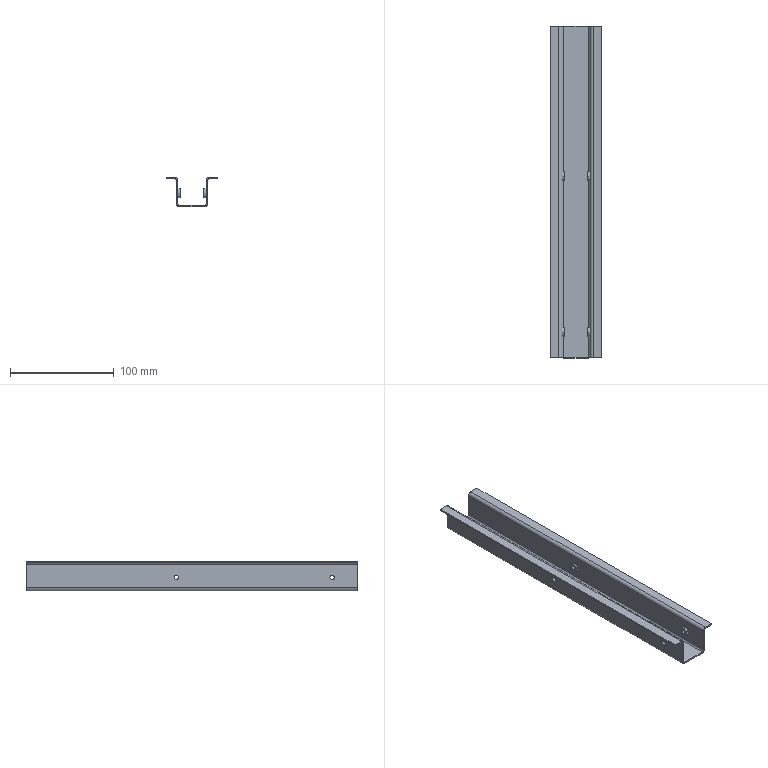Part | SolidWorks | features ICE 2, 3DProfileFeature 1, FlatPattern 1, HoleWzd 1, MirrorPattern 1, SMBaseFlange 1, SheetMetal 1 | 1 solid | 58 faces | box 50 x 320 x 28.5 mm | volume 48347 mm3 | plane 34 | cylinder 24 | commonest cylinder face diameters 4.2 x8 8.7 x8 3 x4 6 x4
STEP:
#1=CARTESIAN_POINT('',(-11.5,-225.,-11.9));
#2=VERTEX_POINT('',#1);
#3=CARTESIAN_POINT('',(-11.5,-225.,-16.1));
#4=VERTEX_POINT('',#3);
#5=CARTESIAN_POINT('',(-11.5,-225.,-14.));
#6=DIRECTION('',(1.,0.,0.));
#7=DIRECTION('',(0.,0.,-1.));
#8=AXIS2_PLACEMENT_3D('',#5,#6,#7);
#9=CIRCLE('',#8,2.1);
#10=EDGE_CURVE('',#2,#4,#9,.T.);
#11=ORIENTED_EDGE('',*,*,#10,.T.);
#12=CARTESIAN_POINT('',(-15.,-225.,-16.1));
#13=VERTEX_POINT('',#12);
#14=CARTESIAN_POINT('',(-15.,-225.,-16.1));
#15=DIRECTION('',(-1.,0.,0.));
#16=VECTOR('',#15,1000.);
#17=LINE('',#14,#16);
#18=EDGE_CURVE('',#4,#13,#17,.T.);
#19=ORIENTED_EDGE('',*,*,#18,.T.);
#20=CARTESIAN_POINT('',(-15.,-225.,-11.9));
#21=VERTEX_POINT('',#20);
#22=CARTESIAN_POINT('',(-15.,-225.,-14.));
#23=DIRECTION('',(-1.,0.,0.));
#24=DIRECTION('',(0.,0.,1.));
#25=AXIS2_PLACEMENT_3D('',#22,#23,#24);
#26=CIRCLE('',#25,2.1);
#27=EDGE_CURVE('',#13,#21,#26,.T.);
#28=ORIENTED_EDGE('',*,*,#27,.T.);
#29=CARTESIAN_POINT('',(-15.,-225.,-11.9));
#30=DIRECTION('',(-1.,0.,0.));
#31=VECTOR('',#30,1000.);
#32=LINE('',#29,#31);
#33=EDGE_CURVE('',#2,#21,#32,.T.);
#34=ORIENTED_EDGE('',*,*,#33,.F.);
#35=EDGE_LOOP('',(#11,#19,#28,#34));
#36=FACE_OUTER_BOUND('',#35,.T.);
#37=CARTESIAN_POINT('',(-15.,-225.,-14.));
#38=DIRECTION('',(-1.,0.,0.));
#39=DIRECTION('',(0.,0.,1.));
#40=AXIS2_PLACEMENT_3D('',#37,#38,#39);
#41=CYLINDRICAL_SURFACE('',#40,2.1);
#42=ADVANCED_FACE('',(#36),#41,.F.);
#43=CARTESIAN_POINT('',(15.,-225.,-11.9));
#44=VERTEX_POINT('',#43);
#45=CARTESIAN_POINT('',(15.,-225.,-16.1));
#46=VERTEX_POINT('',#45);
#47=CARTESIAN_POINT('',(15.,-225.,-14.));
#48=DIRECTION('',(1.,0.,0.));
#49=DIRECTION('',(0.,0.,-1.));
#50=AXIS2_PLACEMENT_3D('',#47,#48,#49);
#51=CIRCLE('',#50,2.1);
#52=EDGE_CURVE('',#44,#46,#51,.T.);
#53=ORIENTED_EDGE('',*,*,#52,.T.);
#54=CARTESIAN_POINT('',(11.5,-225.,-16.1));
#55=VERTEX_POINT('',#54);
#56=CARTESIAN_POINT('',(-15.,-225.,-16.1));
#57=DIRECTION('',(-1.,0.,0.));
#58=VECTOR('',#57,1000.);
#59=LINE('',#56,#58);
#60=EDGE_CURVE('',#46,#55,#59,.T.);
#61=ORIENTED_EDGE('',*,*,#60,.T.);
#62=CARTESIAN_POINT('',(11.5,-225.,-11.9));
#63=VERTEX_POINT('',#62);
#64=CARTESIAN_POINT('',(11.5,-225.,-14.));
#65=DIRECTION('',(-1.,0.,0.));
#66=DIRECTION('',(0.,0.,1.));
#67=AXIS2_PLACEMENT_3D('',#64,#65,#66);
#68=CIRCLE('',#67,2.1);
#69=EDGE_CURVE('',#55,#63,#68,.T.);
#70=ORIENTED_EDGE('',*,*,#69,.T.);
#71=CARTESIAN_POINT('',(-15.,-225.,-11.9));
#72=DIRECTION('',(-1.,0.,0.));
#73=VECTOR('',#72,1000.);
#74=LINE('',#71,#73);
#75=EDGE_CURVE('',#44,#63,#74,.T.);
#76=ORIENTED_EDGE('',*,*,#75,.F.);
#77=EDGE_LOOP('',(#53,#61,#70,#76));
#78=FACE_OUTER_BOUND('',#77,.T.);
#79=CARTESIAN_POINT('',(-15.,-225.,-14.));
#80=DIRECTION('',(-1.,0.,0.));
#81=DIRECTION('',(0.,0.,1.));
#82=AXIS2_PLACEMENT_3D('',#79,#80,#81);
#83=CYLINDRICAL_SURFACE('',#82,2.1);
#84=ADVANCED_FACE('',(#78),#83,.F.);
#85=CARTESIAN_POINT('',(15.,-75.,-11.9));
#86=VERTEX_POINT('',#85);
#87=CARTESIAN_POINT('',(15.,-75.,-16.1));
#88=VERTEX_POINT('',#87);
#89=CARTESIAN_POINT('',(15.,-75.,-14.));
#90=DIRECTION('',(1.,0.,0.));
#91=DIRECTION('',(0.,0.,-1.));
#92=AXIS2_PLACEMENT_3D('',#89,#90,#91);
#93=CIRCLE('',#92,2.1);
#94=EDGE_CURVE('',#86,#88,#93,.T.);
#95=ORIENTED_EDGE('',*,*,#94,.T.);
#96=CARTESIAN_POINT('',(11.5,-75.,-16.1));
#97=VERTEX_POINT('',#96);
#98=CARTESIAN_POINT('',(-15.,-75.,-16.1));
#99=DIRECTION('',(-1.,0.,0.));
#100=VECTOR('',#99,1000.);
#101=LINE('',#98,#100);
#102=EDGE_CURVE('',#88,#97,#101,.T.);
#103=ORIENTED_EDGE('',*,*,#102,.T.);
#104=CARTESIAN_POINT('',(11.5,-75.,-11.9));
#105=VERTEX_POINT('',#104);
#106=CARTESIAN_POINT('',(11.5,-75.,-14.));
#107=DIRECTION('',(1.,0.,0.));
#108=DIRECTION('',(0.,0.,-1.));
#109=AXIS2_PLACEMENT_3D('',#106,#107,#108);
#110=CIRCLE('',#109,2.1);
#111=EDGE_CURVE('',#105,#97,#110,.T.);
#112=ORIENTED_EDGE('',*,*,#111,.F.);
#113=CARTESIAN_POINT('',(-15.,-75.,-11.9));
#114=DIRECTION('',(-1.,0.,0.));
#115=VECTOR('',#114,1000.);
#116=LINE('',#113,#115);
#117=EDGE_CURVE('',#86,#105,#116,.T.);
#118=ORIENTED_EDGE('',*,*,#117,.F.);
#119=EDGE_LOOP('',(#95,#103,#112,#118));
#120=FACE_OUTER_BOUND('',#119,.T.);
#121=CARTESIAN_POINT('',(-15.,-75.,-14.));
#122=DIRECTION('',(-1.,0.,0.));
#123=DIRECTION('',(0.,0.,1.));
#124=AXIS2_PLACEMENT_3D('',#121,#122,#123);
#125=CYLINDRICAL_SURFACE('',#124,2.1);
#126=ADVANCED_FACE('',(#120),#125,.F.);
#127=CARTESIAN_POINT('',(-11.5,-75.,-16.1));
#128=VERTEX_POINT('',#127);
#129=CARTESIAN_POINT('',(-11.5,-75.,-11.9));
#130=VERTEX_POINT('',#129);
#131=CARTESIAN_POINT('',(-11.5,-75.,-14.));
#132=DIRECTION('',(-1.,0.,0.));
#133=DIRECTION('',(0.,0.,1.));
#134=AXIS2_PLACEMENT_3D('',#131,#132,#133);
#135=CIRCLE('',#134,2.1);
#136=EDGE_CURVE('',#128,#130,#135,.T.);
#137=ORIENTED_EDGE('',*,*,#136,.F.);
#138=CARTESIAN_POINT('',(-15.,-75.,-16.1));
#139=VERTEX_POINT('',#138);
#140=CARTESIAN_POINT('',(-15.,-75.,-16.1));
#141=DIRECTION('',(-1.,0.,0.));
#142=VECTOR('',#141,1000.);
#143=LINE('',#140,#142);
#144=EDGE_CURVE('',#128,#139,#143,.T.);
#145=ORIENTED_EDGE('',*,*,#144,.T.);
#146=CARTESIAN_POINT('',(-15.,-75.,-11.9));
#147=VERTEX_POINT('',#146);
#148=CARTESIAN_POINT('',(-15.,-75.,-14.));
#149=DIRECTION('',(-1.,0.,0.));
#150=DIRECTION('',(0.,0.,1.));
#151=AXIS2_PLACEMENT_3D('',#148,#149,#150);
#152=CIRCLE('',#151,2.1);
#153=EDGE_CURVE('',#139,#147,#152,.T.);
#154=ORIENTED_EDGE('',*,*,#153,.T.);
#155=CARTESIAN_POINT('',(-15.,-75.,-11.9));
#156=DIRECTION('',(-1.,0.,0.));
#157=VECTOR('',#156,1000.);
#158=LINE('',#155,#157);
#159=EDGE_CURVE('',#130,#147,#158,.T.);
#160=ORIENTED_EDGE('',*,*,#159,.F.);
#161=EDGE_LOOP('',(#137,#145,#154,#160));
#162=FACE_OUTER_BOUND('',#161,.T.);
#163=CARTESIAN_POINT('',(-15.,-75.,-14.));
#164=DIRECTION('',(-1.,0.,0.));
#165=DIRECTION('',(0.,0.,1.));
#166=AXIS2_PLACEMENT_3D('',#163,#164,#165);
#167=CYLINDRICAL_SURFACE('',#166,2.1);
#168=ADVANCED_FACE('',(#162),#167,.F.);
#169=CARTESIAN_POINT('',(11.5,-75.,-9.65));
#170=VERTEX_POINT('',#169);
#171=CARTESIAN_POINT('',(11.5,-75.,-18.35));
#172=VERTEX_POINT('',#171);
#173=CARTESIAN_POINT('',(11.5,-75.,-14.));
#174=DIRECTION('',(-1.,0.,0.));
#175=DIRECTION('',(0.,0.,1.));
#176=AXIS2_PLACEMENT_3D('',#173,#174,#175);
#177=CIRCLE('',#176,4.35);
#178=EDGE_CURVE('',#170,#172,#177,.T.);
#179=ORIENTED_EDGE('',*,*,#178,.F.);
#180=CARTESIAN_POINT('',(13.5,-75.,-9.65));
#181=VERTEX_POINT('',#180);
#182=CARTESIAN_POINT('',(11.5,-75.,-9.65));
#183=DIRECTION('',(1.,0.,0.));
#184=VECTOR('',#183,1000.);
#185=LINE('',#182,#184);
#186=EDGE_CURVE('',#170,#181,#185,.T.);
#187=ORIENTED_EDGE('',*,*,#186,.T.);
#188=CARTESIAN_POINT('',(13.5,-75.,-18.35));
#189=VERTEX_POINT('',#188);
#190=CARTESIAN_POINT('',(13.5,-75.,-14.));
#191=DIRECTION('',(-1.,0.,0.));
#192=DIRECTION('',(0.,0.,-1.));
#193=AXIS2_PLACEMENT_3D('',#190,#191,#192);
#194=CIRCLE('',#193,4.35);
#195=EDGE_CURVE('',#181,#189,#194,.T.);
#196=ORIENTED_EDGE('',*,*,#195,.T.);
#197=CARTESIAN_POINT('',(11.5,-75.,-18.35));
#198=DIRECTION('',(1.,0.,0.));
#199=VECTOR('',#198,1000.);
#200=LINE('',#197,#199);
#201=EDGE_CURVE('',#172,#189,#200,.T.);
#202=ORIENTED_EDGE('',*,*,#201,.F.);
#203=EDGE_LOOP('',(#179,#187,#196,#202));
#204=FACE_OUTER_BOUND('',#203,.T.);
#205=CARTESIAN_POINT('',(11.5,-75.,-14.));
#206=DIRECTION('',(1.,0.,0.));
#207=DIRECTION('',(0.,0.,-1.));
#208=AXIS2_PLACEMENT_3D('',#205,#206,#207);
#209=CYLINDRICAL_SURFACE('',#208,4.35);
#210=ADVANCED_FACE('',(#204),#209,.T.);
#211=CARTESIAN_POINT('',(11.5,-225.,-9.65));
#212=VERTEX_POINT('',#211);
#213=CARTESIAN_POINT('',(11.5,-225.,-18.35));
#214=VERTEX_POINT('',#213);
#215=CARTESIAN_POINT('',(11.5,-225.,-14.));
#216=DIRECTION('',(-1.,0.,0.));
#217=DIRECTION('',(0.,0.,-1.));
#218=AXIS2_PLACEMENT_3D('',#215,#216,#217);
#219=CIRCLE('',#218,4.35);
#220=EDGE_CURVE('',#212,#214,#219,.T.);
#221=ORIENTED_EDGE('',*,*,#220,.F.);
#222=CARTESIAN_POINT('',(13.5,-225.,-9.65));
#223=VERTEX_POINT('',#222);
#224=CARTESIAN_POINT('',(11.5,-225.,-9.65));
#225=DIRECTION('',(1.,0.,0.));
#226=VECTOR('',#225,1000.);
#227=LINE('',#224,#226);
#228=EDGE_CURVE('',#212,#223,#227,.T.);
#229=ORIENTED_EDGE('',*,*,#228,.T.);
#230=CARTESIAN_POINT('',(13.5,-225.,-18.35));
#231=VERTEX_POINT('',#230);
#232=CARTESIAN_POINT('',(13.5,-225.,-14.));
#233=DIRECTION('',(-1.,0.,0.));
#234=DIRECTION('',(0.,0.,-1.));
#235=AXIS2_PLACEMENT_3D('',#232,#233,#234);
#236=CIRCLE('',#235,4.35);
#237=EDGE_CURVE('',#223,#231,#236,.T.);
#238=ORIENTED_EDGE('',*,*,#237,.T.);
#239=CARTESIAN_POINT('',(11.5,-225.,-18.35));
#240=DIRECTION('',(1.,0.,0.));
#241=VECTOR('',#240,1000.);
#242=LINE('',#239,#241);
#243=EDGE_CURVE('',#214,#231,#242,.T.);
#244=ORIENTED_EDGE('',*,*,#243,.F.);
#245=EDGE_LOOP('',(#221,#229,#238,#244));
#246=FACE_OUTER_BOUND('',#245,.T.);
#247=CARTESIAN_POINT('',(11.5,-225.,-14.));
#248=DIRECTION('',(1.,0.,0.));
#249=DIRECTION('',(0.,0.,-1.));
#250=AXIS2_PLACEMENT_3D('',#247,#248,#249);
#251=CYLINDRICAL_SURFACE('',#250,4.35);
#252=ADVANCED_FACE('',(#246),#251,.T.);
#253=CARTESIAN_POINT('',(-11.5,-75.,-9.65));
#254=VERTEX_POINT('',#253);
#255=CARTESIAN_POINT('',(-11.5,-75.,-18.35));
#256=VERTEX_POINT('',#255);
#257=CARTESIAN_POINT('',(-11.5,-75.,-14.));
#258=DIRECTION('',(-1.,0.,0.));
#259=DIRECTION('',(0.,0.,1.));
#260=AXIS2_PLACEMENT_3D('',#257,#258,#259);
#261=CIRCLE('',#260,4.35);
#262=EDGE_CURVE('',#254,#256,#261,.T.);
#263=ORIENTED_EDGE('',*,*,#262,.T.);
#264=CARTESIAN_POINT('',(-13.5,-75.,-18.35));
#265=VERTEX_POINT('',#264);
#266=CARTESIAN_POINT('',(-11.5,-75.,-18.35));
#267=DIRECTION('',(-1.,0.,0.));
#268=VECTOR('',#267,1000.);
#269=LINE('',#266,#268);
#270=EDGE_CURVE('',#256,#265,#269,.T.);
#271=ORIENTED_EDGE('',*,*,#270,.T.);
#272=CARTESIAN_POINT('',(-13.5,-75.,-9.65));
#273=VERTEX_POINT('',#272);
#274=CARTESIAN_POINT('',(-13.5,-75.,-14.));
#275=DIRECTION('',(-1.,0.,0.));
#276=DIRECTION('',(0.,0.,1.));
#277=AXIS2_PLACEMENT_3D('',#274,#275,#276);
#278=CIRCLE('',#277,4.35);
#279=EDGE_CURVE('',#273,#265,#278,.T.);
#280=ORIENTED_EDGE('',*,*,#279,.F.);
#281=CARTESIAN_POINT('',(-11.5,-75.,-9.65));
#282=DIRECTION('',(-1.,0.,0.));
#283=VECTOR('',#282,1000.);
#284=LINE('',#281,#283);
#285=EDGE_CURVE('',#254,#273,#284,.T.);
#286=ORIENTED_EDGE('',*,*,#285,.F.);
#287=EDGE_LOOP('',(#263,#271,#280,#286));
#288=FACE_OUTER_BOUND('',#287,.T.);
#289=CARTESIAN_POINT('',(-11.5,-75.,-14.));
#290=DIRECTION('',(-1.,0.,0.));
#291=DIRECTION('',(0.,0.,1.));
#292=AXIS2_PLACEMENT_3D('',#289,#290,#291);
#293=CYLINDRICAL_SURFACE('',#292,4.35);
#294=ADVANCED_FACE('',(#288),#293,.T.);
#295=CARTESIAN_POINT('',(-11.5,-225.,-9.65));
#296=VERTEX_POINT('',#295);
#297=CARTESIAN_POINT('',(-11.5,-225.,-18.35));
#298=VERTEX_POINT('',#297);
#299=CARTESIAN_POINT('',(-11.5,-225.,-14.));
#300=DIRECTION('',(-1.,0.,0.));
#301=DIRECTION('',(0.,0.,-1.));
#302=AXIS2_PLACEMENT_3D('',#299,#300,#301);
#303=CIRCLE('',#302,4.35);
#304=EDGE_CURVE('',#296,#298,#303,.T.);
#305=ORIENTED_EDGE('',*,*,#304,.T.);
#306=CARTESIAN_POINT('',(-13.5,-225.,-18.35));
#307=VERTEX_POINT('',#306);
#308=CARTESIAN_POINT('',(-11.5,-225.,-18.35));
#309=DIRECTION('',(-1.,0.,0.));
#310=VECTOR('',#309,1000.);
#311=LINE('',#308,#310);
#312=EDGE_CURVE('',#298,#307,#311,.T.);
#313=ORIENTED_EDGE('',*,*,#312,.T.);
#314=CARTESIAN_POINT('',(-13.5,-225.,-9.65));
#315=VERTEX_POINT('',#314);
#316=CARTESIAN_POINT('',(-13.5,-225.,-14.));
#317=DIRECTION('',(-1.,0.,0.));
#318=DIRECTION('',(0.,0.,-1.));
#319=AXIS2_PLACEMENT_3D('',#316,#317,#318);
#320=CIRCLE('',#319,4.35);
#321=EDGE_CURVE('',#315,#307,#320,.T.);
#322=ORIENTED_EDGE('',*,*,#321,.F.);
#323=CARTESIAN_POINT('',(-11.5,-225.,-9.65));
#324=DIRECTION('',(-1.,0.,0.));
#325=VECTOR('',#324,1000.);
#326=LINE('',#323,#325);
#327=EDGE_CURVE('',#296,#315,#326,.T.);
#328=ORIENTED_EDGE('',*,*,#327,.F.);
#329=EDGE_LOOP('',(#305,#313,#322,#328));
#330=FACE_OUTER_BOUND('',#329,.T.);
#331=CARTESIAN_POINT('',(-11.5,-225.,-14.));
#332=DIRECTION('',(-1.,0.,0.));
#333=DIRECTION('',(0.,0.,1.));
#334=AXIS2_PLACEMENT_3D('',#331,#332,#333);
#335=CYLINDRICAL_SURFACE('',#334,4.35);
#336=ADVANCED_FACE('',(#330),#335,.T.);
#337=CARTESIAN_POINT('',(-16.5,70.,1.5));
#338=VERTEX_POINT('',#337);
#339=CARTESIAN_POINT('',(-25.,70.,1.5));
#340=VERTEX_POINT('',#339);
#341=CARTESIAN_POINT('',(-25.,70.,1.5));
#342=DIRECTION('',(-1.,0.,0.));
#343=VECTOR('',#342,1000.);
#344=LINE('',#341,#343);
#345=EDGE_CURVE('',#338,#340,#344,.T.);
#346=ORIENTED_EDGE('',*,*,#345,.F.);
#347=CARTESIAN_POINT('',(-16.5,70.,0.));
#348=VERTEX_POINT('',#347);
#349=CARTESIAN_POINT('',(-16.5,70.,1.5));
#350=DIRECTION('',(0.,0.,-1.));
#351=VECTOR('',#350,1000.);
#352=LINE('',#349,#351);
#353=EDGE_CURVE('',#338,#348,#352,.T.);
#354=ORIENTED_EDGE('',*,*,#353,.T.);
#355=CARTESIAN_POINT('',(-25.,70.,0.));
#356=VERTEX_POINT('',#355);
#357=CARTESIAN_POINT('',(-25.,70.,0.));
#358=DIRECTION('',(-1.,0.,0.));
#359=VECTOR('',#358,1000.);
#360=LINE('',#357,#359);
#361=EDGE_CURVE('',#348,#356,#360,.T.);
#362=ORIENTED_EDGE('',*,*,#361,.T.);
#363=CARTESIAN_POINT('',(-25.,70.,-43.176));
#364=DIRECTION('',(0.,0.,1.));
#365=VECTOR('',#364,1000.);
#366=LINE('',#363,#365);
#367=EDGE_CURVE('',#356,#340,#366,.T.);
#368=ORIENTED_EDGE('',*,*,#367,.T.);
#369=EDGE_LOOP('',(#346,#354,#362,#368));
#370=FACE_OUTER_BOUND('',#369,.T.);
#371=CARTESIAN_POINT('',(25.,70.,-43.176));
#372=DIRECTION('',(0.,-1.,0.));
#373=DIRECTION('',(0.,0.,-1.));
#374=AXIS2_PLACEMENT_3D('',#371,#372,#373);
#375=PLANE('',#374);
#376=ADVANCED_FACE('',(#370),#375,.F.);
#377=CARTESIAN_POINT('',(-15.,70.,-24.));
#378=VERTEX_POINT('',#377);
#379=CARTESIAN_POINT('',(-15.,70.,-1.5));
#380=VERTEX_POINT('',#379);
#381=CARTESIAN_POINT('',(-15.,70.,0.));
#382=DIRECTION('',(0.,0.,1.));
#383=VECTOR('',#382,1000.);
#384=LINE('',#381,#383);
#385=EDGE_CURVE('',#378,#380,#384,.T.);
#386=ORIENTED_EDGE('',*,*,#385,.T.);
#387=CARTESIAN_POINT('',(-13.5,70.,-1.5));
#388=VERTEX_POINT('',#387);
#389=CARTESIAN_POINT('',(-15.,70.,-1.5));
#390=DIRECTION('',(1.,0.,0.));
#391=VECTOR('',#390,1000.);
#392=LINE('',#389,#391);
#393=EDGE_CURVE('',#380,#388,#392,.T.);
#394=ORIENTED_EDGE('',*,*,#393,.T.);
#395=CARTESIAN_POINT('',(-13.5,70.,-24.));
#396=VERTEX_POINT('',#395);
#397=CARTESIAN_POINT('',(-13.5,70.,0.));
#398=DIRECTION('',(0.,0.,1.));
#399=VECTOR('',#398,1000.);
#400=LINE('',#397,#399);
#401=EDGE_CURVE('',#396,#388,#400,.T.);
#402=ORIENTED_EDGE('',*,*,#401,.F.);
#403=CARTESIAN_POINT('',(-13.5,70.,-24.));
#404=DIRECTION('',(-1.,0.,0.));
#405=VECTOR('',#404,1000.);
#406=LINE('',#403,#405);
#407=EDGE_CURVE('',#396,#378,#406,.T.);
#408=ORIENTED_EDGE('',*,*,#407,.T.);
#409=EDGE_LOOP('',(#386,#394,#402,#408));
#410=FACE_OUTER_BOUND('',#409,.T.);
#411=CARTESIAN_POINT('',(25.,70.,-43.176));
#412=DIRECTION('',(0.,-1.,0.));
#413=DIRECTION('',(0.,0.,-1.));
#414=AXIS2_PLACEMENT_3D('',#411,#412,#413);
#415=PLANE('',#414);
#416=ADVANCED_FACE('',(#410),#415,.F.);
#417=ORIENTED_EDGE('',*,*,#353,.F.);
#418=CARTESIAN_POINT('',(-16.5,70.,-1.5));
#419=DIRECTION('',(0.,-1.,0.));
#420=DIRECTION('',(0.,0.,-1.));
#421=AXIS2_PLACEMENT_3D('',#418,#419,#420);
#422=CIRCLE('',#421,3.);
#423=EDGE_CURVE('',#388,#338,#422,.T.);
#424=ORIENTED_EDGE('',*,*,#423,.F.);
#425=ORIENTED_EDGE('',*,*,#393,.F.);
#426=CARTESIAN_POINT('',(-16.5,70.,-1.5));
#427=DIRECTION('',(0.,-1.,0.));
#428=DIRECTION('',(0.,0.,-1.));
#429=AXIS2_PLACEMENT_3D('',#426,#427,#428);
#430=CIRCLE('',#429,1.5);
#431=EDGE_CURVE('',#380,#348,#430,.T.);
#432=ORIENTED_EDGE('',*,*,#431,.T.);
#433=EDGE_LOOP('',(#417,#424,#425,#432));
#434=FACE_OUTER_BOUND('',#433,.T.);
#435=CARTESIAN_POINT('',(25.,70.,-43.176));
#436=DIRECTION('',(0.,-1.,0.));
#437=DIRECTION('',(0.,0.,-1.));
#438=AXIS2_PLACEMENT_3D('',#435,#436,#437);
#439=PLANE('',#438);
#440=ADVANCED_FACE('',(#434),#439,.F.);
#441=CARTESIAN_POINT('',(12.,70.,-27.));
#442=VERTEX_POINT('',#441);
#443=CARTESIAN_POINT('',(-12.,70.,-27.));
#444=VERTEX_POINT('',#443);
#445=CARTESIAN_POINT('',(-15.,70.,-27.));
#446=DIRECTION('',(-1.,0.,0.));
#447=VECTOR('',#446,1000.);
#448=LINE('',#445,#447);
#449=EDGE_CURVE('',#442,#444,#448,.T.);
#450=ORIENTED_EDGE('',*,*,#449,.T.);
#451=CARTESIAN_POINT('',(-12.,70.,-25.5));
#452=VERTEX_POINT('',#451);
#453=CARTESIAN_POINT('',(-12.,70.,-27.));
#454=DIRECTION('',(0.,0.,1.));
#455=VECTOR('',#454,1000.);
#456=LINE('',#453,#455);
#457=EDGE_CURVE('',#444,#452,#456,.T.);
#458=ORIENTED_EDGE('',*,*,#457,.T.);
#459=CARTESIAN_POINT('',(12.,70.,-25.5));
#460=VERTEX_POINT('',#459);
#461=CARTESIAN_POINT('',(-15.,70.,-25.5));
#462=DIRECTION('',(-1.,0.,0.));
#463=VECTOR('',#462,1000.);
#464=LINE('',#461,#463);
#465=EDGE_CURVE('',#460,#452,#464,.T.);
#466=ORIENTED_EDGE('',*,*,#465,.F.);
#467=CARTESIAN_POINT('',(12.,70.,-25.5));
#468=DIRECTION('',(0.,0.,-1.));
#469=VECTOR('',#468,1000.);
#470=LINE('',#467,#469);
#471=EDGE_CURVE('',#460,#442,#470,.T.);
#472=ORIENTED_EDGE('',*,*,#471,.T.);
#473=EDGE_LOOP('',(#450,#458,#466,#472));
#474=FACE_OUTER_BOUND('',#473,.T.);
#475=CARTESIAN_POINT('',(25.,70.,-43.176));
#476=DIRECTION('',(0.,-1.,0.));
#477=DIRECTION('',(0.,0.,-1.));
#478=AXIS2_PLACEMENT_3D('',#475,#476,#477);
#479=PLANE('',#478);
#480=ADVANCED_FACE('',(#474),#479,.F.);
#481=ORIENTED_EDGE('',*,*,#407,.F.);
#482=CARTESIAN_POINT('',(-12.,70.,-24.));
#483=DIRECTION('',(0.,1.,0.));
#484=DIRECTION('',(0.,0.,-1.));
#485=AXIS2_PLACEMENT_3D('',#482,#483,#484);
#486=CIRCLE('',#485,1.5);
#487=EDGE_CURVE('',#452,#396,#486,.T.);
#488=ORIENTED_EDGE('',*,*,#487,.F.);
#489=ORIENTED_EDGE('',*,*,#457,.F.);
#490=CARTESIAN_POINT('',(-12.,70.,-24.));
#491=DIRECTION('',(0.,1.,0.));
#492=DIRECTION('',(0.,0.,-1.));
#493=AXIS2_PLACEMENT_3D('',#490,#491,#492);
#494=CIRCLE('',#493,3.);
#495=EDGE_CURVE('',#444,#378,#494,.T.);
#496=ORIENTED_EDGE('',*,*,#495,.T.);
#497=EDGE_LOOP('',(#481,#488,#489,#496));
#498=FACE_OUTER_BOUND('',#497,.T.);
#499=CARTESIAN_POINT('',(25.,70.,-43.176));
#500=DIRECTION('',(0.,-1.,0.));
#501=DIRECTION('',(0.,0.,-1.));
#502=AXIS2_PLACEMENT_3D('',#499,#500,#501);
#503=PLANE('',#502);
#504=ADVANCED_FACE('',(#498),#503,.F.);
#505=CARTESIAN_POINT('',(15.,70.,-1.5));
#506=VERTEX_POINT('',#505);
#507=CARTESIAN_POINT('',(15.,70.,-24.));
#508=VERTEX_POINT('',#507);
#509=CARTESIAN_POINT('',(15.,70.,-27.));
#510=DIRECTION('',(0.,0.,-1.));
#511=VECTOR('',#510,1000.);
#512=LINE('',#509,#511);
#513=EDGE_CURVE('',#506,#508,#512,.T.);
#514=ORIENTED_EDGE('',*,*,#513,.T.);
#515=CARTESIAN_POINT('',(13.5,70.,-24.));
#516=VERTEX_POINT('',#515);
#517=CARTESIAN_POINT('',(15.,70.,-24.));
#518=DIRECTION('',(-1.,0.,0.));
#519=VECTOR('',#518,1000.);
#520=LINE('',#517,#519);
#521=EDGE_CURVE('',#508,#516,#520,.T.);
#522=ORIENTED_EDGE('',*,*,#521,.T.);
#523=CARTESIAN_POINT('',(13.5,70.,-1.5));
#524=VERTEX_POINT('',#523);
#525=CARTESIAN_POINT('',(13.5,70.,-27.));
#526=DIRECTION('',(0.,0.,-1.));
#527=VECTOR('',#526,1000.);
#528=LINE('',#525,#527);
#529=EDGE_CURVE('',#524,#516,#528,.T.);
#530=ORIENTED_EDGE('',*,*,#529,.F.);
#531=CARTESIAN_POINT('',(13.5,70.,-1.5));
#532=DIRECTION('',(1.,0.,0.));
#533=VECTOR('',#532,1000.);
#534=LINE('',#531,#533);
#535=EDGE_CURVE('',#524,#506,#534,.T.);
#536=ORIENTED_EDGE('',*,*,#535,.T.);
#537=EDGE_LOOP('',(#514,#522,#530,#536));
#538=FACE_OUTER_BOUND('',#537,.T.);
#539=CARTESIAN_POINT('',(25.,70.,-43.176));
#540=DIRECTION('',(0.,-1.,0.));
#541=DIRECTION('',(0.,0.,-1.));
#542=AXIS2_PLACEMENT_3D('',#539,#540,#541);
#543=PLANE('',#542);
#544=ADVANCED_FACE('',(#538),#543,.F.);
#545=ORIENTED_EDGE('',*,*,#471,.F.);
#546=CARTESIAN_POINT('',(12.,70.,-24.));
#547=DIRECTION('',(0.,1.,0.));
#548=DIRECTION('',(0.,0.,-1.));
#549=AXIS2_PLACEMENT_3D('',#546,#547,#548);
#550=CIRCLE('',#549,1.5);
#551=EDGE_CURVE('',#516,#460,#550,.T.);
#552=ORIENTED_EDGE('',*,*,#551,.F.);
#553=ORIENTED_EDGE('',*,*,#521,.F.);
#554=CARTESIAN_POINT('',(12.,70.,-24.));
#555=DIRECTION('',(0.,1.,0.));
#556=DIRECTION('',(0.,0.,-1.));
#557=AXIS2_PLACEMENT_3D('',#554,#555,#556);
#558=CIRCLE('',#557,3.);
#559=EDGE_CURVE('',#508,#442,#558,.T.);
#560=ORIENTED_EDGE('',*,*,#559,.T.);
#561=EDGE_LOOP('',(#545,#552,#553,#560));
#562=FACE_OUTER_BOUND('',#561,.T.);
#563=CARTESIAN_POINT('',(25.,70.,-43.176));
#564=DIRECTION('',(0.,-1.,0.));
#565=DIRECTION('',(0.,0.,-1.));
#566=AXIS2_PLACEMENT_3D('',#563,#564,#565);
#567=PLANE('',#566);
#568=ADVANCED_FACE('',(#562),#567,.F.);
#569=CARTESIAN_POINT('',(25.,70.,0.));
#570=VERTEX_POINT('',#569);
#571=CARTESIAN_POINT('',(16.5,70.,0.));
#572=VERTEX_POINT('',#571);
#573=CARTESIAN_POINT('',(15.,70.,0.));
#574=DIRECTION('',(-1.,0.,0.));
#575=VECTOR('',#574,1000.);
#576=LINE('',#573,#575);
#577=EDGE_CURVE('',#570,#572,#576,.T.);
#578=ORIENTED_EDGE('',*,*,#577,.T.);
#579=CARTESIAN_POINT('',(16.5,70.,1.5));
#580=VERTEX_POINT('',#579);
#581=CARTESIAN_POINT('',(16.5,70.,0.));
#582=DIRECTION('',(0.,0.,1.));
#583=VECTOR('',#582,1000.);
#584=LINE('',#581,#583);
#585=EDGE_CURVE('',#572,#580,#584,.T.);
#586=ORIENTED_EDGE('',*,*,#585,.T.);
#587=CARTESIAN_POINT('',(25.,70.,1.5));
#588=VERTEX_POINT('',#587);
#589=CARTESIAN_POINT('',(15.,70.,1.5));
#590=DIRECTION('',(-1.,0.,0.));
#591=VECTOR('',#590,1000.);
#592=LINE('',#589,#591);
#593=EDGE_CURVE('',#588,#580,#592,.T.);
#594=ORIENTED_EDGE('',*,*,#593,.F.);
#595=CARTESIAN_POINT('',(25.,70.,-43.176));
#596=DIRECTION('',(0.,0.,1.));
#597=VECTOR('',#596,1000.);
#598=LINE('',#595,#597);
#599=EDGE_CURVE('',#570,#588,#598,.T.);
#600=ORIENTED_EDGE('',*,*,#599,.F.);
#601=EDGE_LOOP('',(#578,#586,#594,#600));
#602=FACE_OUTER_BOUND('',#601,.T.);
#603=CARTESIAN_POINT('',(25.,70.,-43.176));
#604=DIRECTION('',(0.,-1.,0.));
#605=DIRECTION('',(0.,0.,-1.));
#606=AXIS2_PLACEMENT_3D('',#603,#604,#605);
#607=PLANE('',#606);
#608=ADVANCED_FACE('',(#602),#607,.F.);
#609=CARTESIAN_POINT('',(-16.5,-250.,0.));
#610=VERTEX_POINT('',#609);
#611=CARTESIAN_POINT('',(-16.5,-250.,1.5));
#612=VERTEX_POINT('',#611);
#613=CARTESIAN_POINT('',(-16.5,-250.,0.));
#614=DIRECTION('',(0.,0.,1.));
#615=VECTOR('',#614,1000.);
#616=LINE('',#613,#615);
#617=EDGE_CURVE('',#610,#612,#616,.T.);
#618=ORIENTED_EDGE('',*,*,#617,.F.);
#619=CARTESIAN_POINT('',(-15.,-250.,-1.5));
#620=VERTEX_POINT('',#619);
#621=CARTESIAN_POINT('',(-16.5,-250.,-1.5));
#622=DIRECTION('',(0.,1.,0.));
#623=DIRECTION('',(0.,0.,-1.));
#624=AXIS2_PLACEMENT_3D('',#621,#622,#623);
#625=CIRCLE('',#624,1.5);
#626=EDGE_CURVE('',#610,#620,#625,.T.);
#627=ORIENTED_EDGE('',*,*,#626,.T.);
#628=CARTESIAN_POINT('',(-13.5,-250.,-1.5));
#629=VERTEX_POINT('',#628);
#630=CARTESIAN_POINT('',(-13.5,-250.,-1.5));
#631=DIRECTION('',(-1.,0.,0.));
#632=VECTOR('',#631,1000.);
#633=LINE('',#630,#632);
#634=EDGE_CURVE('',#629,#620,#633,.T.);
#635=ORIENTED_EDGE('',*,*,#634,.F.);
#636=CARTESIAN_POINT('',(-16.5,-250.,-1.5));
#637=DIRECTION('',(0.,1.,0.));
#638=DIRECTION('',(1.,0.,0.));
#639=AXIS2_PLACEMENT_3D('',#636,#637,#638);
#640=CIRCLE('',#639,3.);
#641=EDGE_CURVE('',#612,#629,#640,.T.);
#642=ORIENTED_EDGE('',*,*,#641,.F.);
#643=EDGE_LOOP('',(#618,#627,#635,#642));
#644=FACE_OUTER_BOUND('',#643,.T.);
#645=CARTESIAN_POINT('',(-16.5,-250.,0.));
#646=DIRECTION('',(0.,-1.,0.));
#647=DIRECTION('',(0.,0.,-1.));
#648=AXIS2_PLACEMENT_3D('',#645,#646,#647);
#649=PLANE('',#648);
#650=ADVANCED_FACE('',(#644),#649,.T.);
#651=CARTESIAN_POINT('',(-25.,-250.,0.));
#652=VERTEX_POINT('',#651);
#653=CARTESIAN_POINT('',(-25.,-250.,0.));
#654=DIRECTION('',(1.,0.,0.));
#655=VECTOR('',#654,1000.);
#656=LINE('',#653,#655);
#657=EDGE_CURVE('',#652,#610,#656,.T.);
#658=ORIENTED_EDGE('',*,*,#657,.T.);
#659=ORIENTED_EDGE('',*,*,#617,.T.);
#660=CARTESIAN_POINT('',(-25.,-250.,1.5));
#661=VERTEX_POINT('',#660);
#662=CARTESIAN_POINT('',(-25.,-250.,1.5));
#663=DIRECTION('',(1.,0.,0.));
#664=VECTOR('',#663,1000.);
#665=LINE('',#662,#664);
#666=EDGE_CURVE('',#661,#612,#665,.T.);
#667=ORIENTED_EDGE('',*,*,#666,.F.);
#668=CARTESIAN_POINT('',(-25.,-250.,1.5));
#669=DIRECTION('',(0.,0.,-1.));
#670=VECTOR('',#669,1000.);
#671=LINE('',#668,#670);
#672=EDGE_CURVE('',#661,#652,#671,.T.);
#673=ORIENTED_EDGE('',*,*,#672,.T.);
#674=EDGE_LOOP('',(#658,#659,#667,#673));
#675=FACE_OUTER_BOUND('',#674,.T.);
#676=CARTESIAN_POINT('',(-13.5,-250.,-1.5));
#677=DIRECTION('',(0.,-1.,0.));
#678=DIRECTION('',(0.,0.,-1.));
#679=AXIS2_PLACEMENT_3D('',#676,#677,#678);
#680=PLANE('',#679);
#681=ADVANCED_FACE('',(#675),#680,.T.);
#682=CARTESIAN_POINT('',(-15.,-250.,-24.));
#683=VERTEX_POINT('',#682);
#684=CARTESIAN_POINT('',(-13.5,-250.,-24.));
#685=VERTEX_POINT('',#684);
#686=CARTESIAN_POINT('',(-15.,-250.,-24.));
#687=DIRECTION('',(1.,0.,0.));
#688=VECTOR('',#687,1000.);
#689=LINE('',#686,#688);
#690=EDGE_CURVE('',#683,#685,#689,.T.);
#691=ORIENTED_EDGE('',*,*,#690,.F.);
#692=CARTESIAN_POINT('',(-12.,-250.,-27.));
#693=VERTEX_POINT('',#692);
#694=CARTESIAN_POINT('',(-12.,-250.,-24.));
#695=DIRECTION('',(0.,-1.,0.));
#696=DIRECTION('',(0.,0.,1.));
#697=AXIS2_PLACEMENT_3D('',#694,#695,#696);
#698=CIRCLE('',#697,3.);
#699=EDGE_CURVE('',#683,#693,#698,.T.);
#700=ORIENTED_EDGE('',*,*,#699,.T.);
#701=CARTESIAN_POINT('',(-12.,-250.,-25.5));
#702=VERTEX_POINT('',#701);
#703=CARTESIAN_POINT('',(-12.,-250.,-25.5));
#704=DIRECTION('',(0.,0.,-1.));
#705=VECTOR('',#704,1000.);
#706=LINE('',#703,#705);
#707=EDGE_CURVE('',#702,#693,#706,.T.);
#708=ORIENTED_EDGE('',*,*,#707,.F.);
#709=CARTESIAN_POINT('',(-12.,-250.,-24.));
#710=DIRECTION('',(0.,-1.,0.));
#711=DIRECTION('',(1.,0.,0.));
#712=AXIS2_PLACEMENT_3D('',#709,#710,#711);
#713=CIRCLE('',#712,1.5);
#714=EDGE_CURVE('',#685,#702,#713,.T.);
#715=ORIENTED_EDGE('',*,*,#714,.F.);
#716=EDGE_LOOP('',(#691,#700,#708,#715));
#717=FACE_OUTER_BOUND('',#716,.T.);
#718=CARTESIAN_POINT('',(-15.,-250.,-24.));
#719=DIRECTION('',(0.,-1.,0.));
#720=DIRECTION('',(0.,0.,-1.));
#721=AXIS2_PLACEMENT_3D('',#718,#719,#720);
#722=PLANE('',#721);
#723=ADVANCED_FACE('',(#717),#722,.T.);
#724=CARTESIAN_POINT('',(-15.,-250.,0.));
#725=DIRECTION('',(0.,0.,-1.));
#726=VECTOR('',#725,1000.);
#727=LINE('',#724,#726);
#728=EDGE_CURVE('',#620,#683,#727,.T.);
#729=ORIENTED_EDGE('',*,*,#728,.T.);
#730=ORIENTED_EDGE('',*,*,#690,.T.);
#731=CARTESIAN_POINT('',(-13.5,-250.,0.));
#732=DIRECTION('',(0.,0.,-1.));
#733=VECTOR('',#732,1000.);
#734=LINE('',#731,#733);
#735=EDGE_CURVE('',#629,#685,#734,.T.);
#736=ORIENTED_EDGE('',*,*,#735,.F.);
#737=ORIENTED_EDGE('',*,*,#634,.T.);
#738=EDGE_LOOP('',(#729,#730,#736,#737));
#739=FACE_OUTER_BOUND('',#738,.T.);
#740=CARTESIAN_POINT('',(-12.,-250.,-25.5));
#741=DIRECTION('',(0.,-1.,0.));
#742=DIRECTION('',(0.,0.,-1.));
#743=AXIS2_PLACEMENT_3D('',#740,#741,#742);
#744=PLANE('',#743);
#745=ADVANCED_FACE('',(#739),#744,.T.);
#746=CARTESIAN_POINT('',(12.,-250.,-27.));
#747=VERTEX_POINT('',#746);
#748=CARTESIAN_POINT('',(12.,-250.,-25.5));
#749=VERTEX_POINT('',#748);
#750=CARTESIAN_POINT('',(12.,-250.,-27.));
#751=DIRECTION('',(0.,0.,1.));
#752=VECTOR('',#751,1000.);
#753=LINE('',#750,#752);
#754=EDGE_CURVE('',#747,#749,#753,.T.);
#755=ORIENTED_EDGE('',*,*,#754,.F.);
#756=CARTESIAN_POINT('',(15.,-250.,-24.));
#757=VERTEX_POINT('',#756);
#758=CARTESIAN_POINT('',(12.,-250.,-24.));
#759=DIRECTION('',(0.,-1.,0.));
#760=DIRECTION('',(0.,0.,1.));
#761=AXIS2_PLACEMENT_3D('',#758,#759,#760);
#762=CIRCLE('',#761,3.);
#763=EDGE_CURVE('',#747,#757,#762,.T.);
#764=ORIENTED_EDGE('',*,*,#763,.T.);
#765=CARTESIAN_POINT('',(13.5,-250.,-24.));
#766=VERTEX_POINT('',#765);
#767=CARTESIAN_POINT('',(13.5,-250.,-24.));
#768=DIRECTION('',(1.,0.,0.));
#769=VECTOR('',#768,1000.);
#770=LINE('',#767,#769);
#771=EDGE_CURVE('',#766,#757,#770,.T.);
#772=ORIENTED_EDGE('',*,*,#771,.F.);
#773=CARTESIAN_POINT('',(12.,-250.,-24.));
#774=DIRECTION('',(0.,-1.,0.));
#775=DIRECTION('',(1.,0.,0.));
#776=AXIS2_PLACEMENT_3D('',#773,#774,#775);
#777=CIRCLE('',#776,1.5);
#778=EDGE_CURVE('',#749,#766,#777,.T.);
#779=ORIENTED_EDGE('',*,*,#778,.F.);
#780=EDGE_LOOP('',(#755,#764,#772,#779));
#781=FACE_OUTER_BOUND('',#780,.T.);
#782=CARTESIAN_POINT('',(12.,-250.,-27.));
#783=DIRECTION('',(0.,-1.,0.));
#784=DIRECTION('',(0.,0.,-1.));
#785=AXIS2_PLACEMENT_3D('',#782,#783,#784);
#786=PLANE('',#785);
#787=ADVANCED_FACE('',(#781),#786,.T.);
#788=CARTESIAN_POINT('',(-15.,-250.,-27.));
#789=DIRECTION('',(1.,0.,0.));
#790=VECTOR('',#789,1000.);
#791=LINE('',#788,#790);
#792=EDGE_CURVE('',#693,#747,#791,.T.);
#793=ORIENTED_EDGE('',*,*,#792,.T.);
#794=ORIENTED_EDGE('',*,*,#754,.T.);
#795=CARTESIAN_POINT('',(-15.,-250.,-25.5));
#796=DIRECTION('',(1.,0.,0.));
#797=VECTOR('',#796,1000.);
#798=LINE('',#795,#797);
#799=EDGE_CURVE('',#702,#749,#798,.T.);
#800=ORIENTED_EDGE('',*,*,#799,.F.);
#801=ORIENTED_EDGE('',*,*,#707,.T.);
#802=EDGE_LOOP('',(#793,#794,#800,#801));
#803=FACE_OUTER_BOUND('',#802,.T.);
#804=CARTESIAN_POINT('',(13.5,-250.,-24.));
#805=DIRECTION('',(0.,-1.,0.));
#806=DIRECTION('',(0.,0.,-1.));
#807=AXIS2_PLACEMENT_3D('',#804,#805,#806);
#808=PLANE('',#807);
#809=ADVANCED_FACE('',(#803),#808,.T.);
#810=CARTESIAN_POINT('',(15.,-250.,-1.5));
#811=VERTEX_POINT('',#810);
#812=CARTESIAN_POINT('',(13.5,-250.,-1.5));
#813=VERTEX_POINT('',#812);
#814=CARTESIAN_POINT('',(15.,-250.,-1.5));
#815=DIRECTION('',(-1.,0.,0.));
#816=VECTOR('',#815,1000.);
#817=LINE('',#814,#816);
#818=EDGE_CURVE('',#811,#813,#817,.T.);
#819=ORIENTED_EDGE('',*,*,#818,.F.);
#820=CARTESIAN_POINT('',(16.5,-250.,0.));
#821=VERTEX_POINT('',#820);
#822=CARTESIAN_POINT('',(16.5,-250.,-1.5));
#823=DIRECTION('',(0.,1.,0.));
#824=DIRECTION('',(0.,0.,-1.));
#825=AXIS2_PLACEMENT_3D('',#822,#823,#824);
#826=CIRCLE('',#825,1.5);
#827=EDGE_CURVE('',#811,#821,#826,.T.);
#828=ORIENTED_EDGE('',*,*,#827,.T.);
#829=CARTESIAN_POINT('',(16.5,-250.,1.5));
#830=VERTEX_POINT('',#829);
#831=CARTESIAN_POINT('',(16.5,-250.,1.5));
#832=DIRECTION('',(0.,0.,-1.));
#833=VECTOR('',#832,1000.);
#834=LINE('',#831,#833);
#835=EDGE_CURVE('',#830,#821,#834,.T.);
#836=ORIENTED_EDGE('',*,*,#835,.F.);
#837=CARTESIAN_POINT('',(16.5,-250.,-1.5));
#838=DIRECTION('',(0.,1.,0.));
#839=DIRECTION('',(1.,0.,0.));
#840=AXIS2_PLACEMENT_3D('',#837,#838,#839);
#841=CIRCLE('',#840,3.);
#842=EDGE_CURVE('',#813,#830,#841,.T.);
#843=ORIENTED_EDGE('',*,*,#842,.F.);
#844=EDGE_LOOP('',(#819,#828,#836,#843));
#845=FACE_OUTER_BOUND('',#844,.T.);
#846=CARTESIAN_POINT('',(15.,-250.,-1.5));
#847=DIRECTION('',(0.,-1.,0.));
#848=DIRECTION('',(0.,0.,-1.));
#849=AXIS2_PLACEMENT_3D('',#846,#847,#848);
#850=PLANE('',#849);
#851=ADVANCED_FACE('',(#845),#850,.T.);
#852=CARTESIAN_POINT('',(15.,-250.,-27.));
#853=DIRECTION('',(0.,0.,1.));
#854=VECTOR('',#853,1000.);
#855=LINE('',#852,#854);
#856=EDGE_CURVE('',#757,#811,#855,.T.);
#857=ORIENTED_EDGE('',*,*,#856,.T.);
#858=ORIENTED_EDGE('',*,*,#818,.T.);
#859=CARTESIAN_POINT('',(13.5,-250.,-27.));
#860=DIRECTION('',(0.,0.,1.));
#861=VECTOR('',#860,1000.);
#862=LINE('',#859,#861);
#863=EDGE_CURVE('',#766,#813,#862,.T.);
#864=ORIENTED_EDGE('',*,*,#863,.F.);
#865=ORIENTED_EDGE('',*,*,#771,.T.);
#866=EDGE_LOOP('',(#857,#858,#864,#865));
#867=FACE_OUTER_BOUND('',#866,.T.);
#868=CARTESIAN_POINT('',(16.5,-250.,1.5));
#869=DIRECTION('',(0.,-1.,0.));
#870=DIRECTION('',(0.,0.,-1.));
#871=AXIS2_PLACEMENT_3D('',#868,#869,#870);
#872=PLANE('',#871);
#873=ADVANCED_FACE('',(#867),#872,.T.);
#874=CARTESIAN_POINT('',(25.,-250.,1.5));
#875=VERTEX_POINT('',#874);
#876=CARTESIAN_POINT('',(25.,250.,1.5));
#877=DIRECTION('',(0.,-1.,0.));
#878=VECTOR('',#877,1000.);
#879=LINE('',#876,#878);
#880=EDGE_CURVE('',#588,#875,#879,.T.);
#881=ORIENTED_EDGE('',*,*,#880,.F.);
#882=ORIENTED_EDGE('',*,*,#593,.T.);
#883=CARTESIAN_POINT('',(16.5,250.,1.5));
#884=DIRECTION('',(0.,-1.,0.));
#885=VECTOR('',#884,1000.);
#886=LINE('',#883,#885);
#887=EDGE_CURVE('',#580,#830,#886,.T.);
#888=ORIENTED_EDGE('',*,*,#887,.T.);
#889=CARTESIAN_POINT('',(15.,-250.,1.5));
#890=DIRECTION('',(1.,0.,0.));
#891=VECTOR('',#890,1000.);
#892=LINE('',#889,#891);
#893=EDGE_CURVE('',#830,#875,#892,.T.);
#894=ORIENTED_EDGE('',*,*,#893,.T.);
#895=EDGE_LOOP('',(#881,#882,#888,#894));
#896=FACE_OUTER_BOUND('',#895,.T.);
#897=CARTESIAN_POINT('',(15.,250.,1.5));
#898=DIRECTION('',(0.,0.,-1.));
#899=DIRECTION('',(-1.,0.,0.));
#900=AXIS2_PLACEMENT_3D('',#897,#898,#899);
#901=PLANE('',#900);
#902=ADVANCED_FACE('',(#896),#901,.F.);
#903=ORIENTED_EDGE('',*,*,#599,.T.);
#904=ORIENTED_EDGE('',*,*,#880,.T.);
#905=CARTESIAN_POINT('',(25.,-250.,0.));
#906=VERTEX_POINT('',#905);
#907=CARTESIAN_POINT('',(25.,-250.,0.));
#908=DIRECTION('',(0.,0.,1.));
#909=VECTOR('',#908,1000.);
#910=LINE('',#907,#909);
#911=EDGE_CURVE('',#906,#875,#910,.T.);
#912=ORIENTED_EDGE('',*,*,#911,.F.);
#913=CARTESIAN_POINT('',(25.,250.,0.));
#914=DIRECTION('',(0.,-1.,0.));
#915=VECTOR('',#914,1000.);
#916=LINE('',#913,#915);
#917=EDGE_CURVE('',#570,#906,#916,.T.);
#918=ORIENTED_EDGE('',*,*,#917,.F.);
#919=EDGE_LOOP('',(#903,#904,#912,#918));
#920=FACE_OUTER_BOUND('',#919,.T.);
#921=CARTESIAN_POINT('',(25.,250.,0.));
#922=DIRECTION('',(1.,0.,0.));
#923=DIRECTION('',(0.,0.,-1.));
#924=AXIS2_PLACEMENT_3D('',#921,#922,#923);
#925=PLANE('',#924);
#926=ADVANCED_FACE('',(#920),#925,.T.);
#927=ORIENTED_EDGE('',*,*,#577,.F.);
#928=ORIENTED_EDGE('',*,*,#917,.T.);
#929=CARTESIAN_POINT('',(15.,-250.,0.));
#930=DIRECTION('',(1.,0.,0.));
#931=VECTOR('',#930,1000.);
#932=LINE('',#929,#931);
#933=EDGE_CURVE('',#821,#906,#932,.T.);
#934=ORIENTED_EDGE('',*,*,#933,.F.);
#935=CARTESIAN_POINT('',(16.5,250.,0.));
#936=DIRECTION('',(0.,-1.,0.));
#937=VECTOR('',#936,1000.);
#938=LINE('',#935,#937);
#939=EDGE_CURVE('',#572,#821,#938,.T.);
#940=ORIENTED_EDGE('',*,*,#939,.F.);
#941=EDGE_LOOP('',(#927,#928,#934,#940));
#942=FACE_OUTER_BOUND('',#941,.T.);
#943=CARTESIAN_POINT('',(15.,250.,0.));
#944=DIRECTION('',(0.,0.,-1.));
#945=DIRECTION('',(-1.,0.,0.));
#946=AXIS2_PLACEMENT_3D('',#943,#944,#945);
#947=PLANE('',#946);
#948=ADVANCED_FACE('',(#942),#947,.T.);
#949=CARTESIAN_POINT('',(16.5,70.,-1.5));
#950=DIRECTION('',(0.,-1.,0.));
#951=DIRECTION('',(0.,0.,-1.));
#952=AXIS2_PLACEMENT_3D('',#949,#950,#951);
#953=CIRCLE('',#952,1.5);
#954=EDGE_CURVE('',#572,#506,#953,.T.);
#955=ORIENTED_EDGE('',*,*,#954,.F.);
#956=ORIENTED_EDGE('',*,*,#939,.T.);
#957=ORIENTED_EDGE('',*,*,#827,.F.);
#958=CARTESIAN_POINT('',(15.,250.,-1.5));
#959=DIRECTION('',(0.,-1.,0.));
#960=VECTOR('',#959,1000.);
#961=LINE('',#958,#960);
#962=EDGE_CURVE('',#506,#811,#961,.T.);
#963=ORIENTED_EDGE('',*,*,#962,.F.);
#964=EDGE_LOOP('',(#955,#956,#957,#963));
#965=FACE_OUTER_BOUND('',#964,.T.);
#966=CARTESIAN_POINT('',(16.5,250.,-1.5));
#967=DIRECTION('',(0.,-1.,0.));
#968=DIRECTION('',(0.,0.,-1.));
#969=AXIS2_PLACEMENT_3D('',#966,#967,#968);
#970=CYLINDRICAL_SURFACE('',#969,1.5);
#971=ADVANCED_FACE('',(#965),#970,.F.);
#972=ORIENTED_EDGE('',*,*,#513,.F.);
#973=ORIENTED_EDGE('',*,*,#962,.T.);
#974=ORIENTED_EDGE('',*,*,#856,.F.);
#975=CARTESIAN_POINT('',(15.,250.,-24.));
#976=DIRECTION('',(0.,-1.,0.));
#977=VECTOR('',#976,1000.);
#978=LINE('',#975,#977);
#979=EDGE_CURVE('',#508,#757,#978,.T.);
#980=ORIENTED_EDGE('',*,*,#979,.F.);
#981=EDGE_LOOP('',(#972,#973,#974,#980));
#982=FACE_OUTER_BOUND('',#981,.T.);
#983=ORIENTED_EDGE('',*,*,#52,.F.);
#984=CARTESIAN_POINT('',(15.,-225.,-14.));
#985=DIRECTION('',(1.,0.,0.));
#986=DIRECTION('',(0.,0.,-1.));
#987=AXIS2_PLACEMENT_3D('',#984,#985,#986);
#988=CIRCLE('',#987,2.1);
#989=EDGE_CURVE('',#46,#44,#988,.T.);
#990=ORIENTED_EDGE('',*,*,#989,.F.);
#991=EDGE_LOOP('',(#983,#990));
#992=FACE_BOUND('',#991,.T.);
#993=ORIENTED_EDGE('',*,*,#94,.F.);
#994=CARTESIAN_POINT('',(15.,-75.,-14.));
#995=DIRECTION('',(1.,0.,0.));
#996=DIRECTION('',(0.,0.,-1.));
#997=AXIS2_PLACEMENT_3D('',#994,#995,#996);
#998=CIRCLE('',#997,2.1);
#999=EDGE_CURVE('',#88,#86,#998,.T.);
#1000=ORIENTED_EDGE('',*,*,#999,.F.);
#1001=EDGE_LOOP('',(#993,#1000));
#1002=FACE_BOUND('',#1001,.T.);
#1003=CARTESIAN_POINT('',(15.,250.,-27.));
#1004=DIRECTION('',(1.,0.,0.));
#1005=DIRECTION('',(0.,0.,-1.));
#1006=AXIS2_PLACEMENT_3D('',#1003,#1004,#1005);
#1007=PLANE('',#1006);
#1008=ADVANCED_FACE('',(#982,#992,#1002),#1007,.T.);
#1009=ORIENTED_EDGE('',*,*,#559,.F.);
#1010=ORIENTED_EDGE('',*,*,#979,.T.);
#1011=ORIENTED_EDGE('',*,*,#763,.F.);
#1012=CARTESIAN_POINT('',(12.,250.,-27.));
#1013=DIRECTION('',(0.,-1.,0.));
#1014=VECTOR('',#1013,1000.);
#1015=LINE('',#1012,#1014);
#1016=EDGE_CURVE('',#442,#747,#1015,.T.);
#1017=ORIENTED_EDGE('',*,*,#1016,.F.);
#1018=EDGE_LOOP('',(#1009,#1010,#1011,#1017));
#1019=FACE_OUTER_BOUND('',#1018,.T.);
#1020=CARTESIAN_POINT('',(12.,250.,-24.));
#1021=DIRECTION('',(0.,-1.,0.));
#1022=DIRECTION('',(0.,0.,-1.));
#1023=AXIS2_PLACEMENT_3D('',#1020,#1021,#1022);
#1024=CYLINDRICAL_SURFACE('',#1023,3.);
#1025=ADVANCED_FACE('',(#1019),#1024,.T.);
#1026=ORIENTED_EDGE('',*,*,#449,.F.);
#1027=ORIENTED_EDGE('',*,*,#1016,.T.);
#1028=ORIENTED_EDGE('',*,*,#792,.F.);
#1029=CARTESIAN_POINT('',(-12.,250.,-27.));
#1030=DIRECTION('',(0.,-1.,0.));
#1031=VECTOR('',#1030,1000.);
#1032=LINE('',#1029,#1031);
#1033=EDGE_CURVE('',#444,#693,#1032,.T.);
#1034=ORIENTED_EDGE('',*,*,#1033,.F.);
#1035=EDGE_LOOP('',(#1026,#1027,#1028,#1034));
#1036=FACE_OUTER_BOUND('',#1035,.T.);
#1037=CARTESIAN_POINT('',(-15.,250.,-27.));
#1038=DIRECTION('',(0.,0.,-1.));
#1039=DIRECTION('',(-1.,0.,0.));
#1040=AXIS2_PLACEMENT_3D('',#1037,#1038,#1039);
#1041=PLANE('',#1040);
#1042=ADVANCED_FACE('',(#1036),#1041,.T.);
#1043=ORIENTED_EDGE('',*,*,#495,.F.);
#1044=ORIENTED_EDGE('',*,*,#1033,.T.);
#1045=ORIENTED_EDGE('',*,*,#699,.F.);
#1046=CARTESIAN_POINT('',(-15.,250.,-24.));
#1047=DIRECTION('',(0.,-1.,0.));
#1048=VECTOR('',#1047,1000.);
#1049=LINE('',#1046,#1048);
#1050=EDGE_CURVE('',#378,#683,#1049,.T.);
#1051=ORIENTED_EDGE('',*,*,#1050,.F.);
#1052=EDGE_LOOP('',(#1043,#1044,#1045,#1051));
#1053=FACE_OUTER_BOUND('',#1052,.T.);
#1054=CARTESIAN_POINT('',(-12.,250.,-24.));
#1055=DIRECTION('',(0.,-1.,0.));
#1056=DIRECTION('',(0.,0.,-1.));
#1057=AXIS2_PLACEMENT_3D('',#1054,#1055,#1056);
#1058=CYLINDRICAL_SURFACE('',#1057,3.);
#1059=ADVANCED_FACE('',(#1053),#1058,.T.);
#1060=ORIENTED_EDGE('',*,*,#385,.F.);
#1061=ORIENTED_EDGE('',*,*,#1050,.T.);
#1062=ORIENTED_EDGE('',*,*,#728,.F.);
#1063=CARTESIAN_POINT('',(-15.,250.,-1.5));
#1064=DIRECTION('',(0.,-1.,0.));
#1065=VECTOR('',#1064,1000.);
#1066=LINE('',#1063,#1065);
#1067=EDGE_CURVE('',#380,#620,#1066,.T.);
#1068=ORIENTED_EDGE('',*,*,#1067,.F.);
#1069=EDGE_LOOP('',(#1060,#1061,#1062,#1068));
#1070=FACE_OUTER_BOUND('',#1069,.T.);
#1071=CARTESIAN_POINT('',(-15.,-225.,-14.));
#1072=DIRECTION('',(-1.,0.,0.));
#1073=DIRECTION('',(0.,0.,1.));
#1074=AXIS2_PLACEMENT_3D('',#1071,#1072,#1073);
#1075=CIRCLE('',#1074,2.1);
#1076=EDGE_CURVE('',#21,#13,#1075,.T.);
#1077=ORIENTED_EDGE('',*,*,#1076,.F.);
#1078=ORIENTED_EDGE('',*,*,#27,.F.);
#1079=EDGE_LOOP('',(#1077,#1078));
#1080=FACE_BOUND('',#1079,.T.);
#1081=CARTESIAN_POINT('',(-15.,-75.,-14.));
#1082=DIRECTION('',(-1.,0.,0.));
#1083=DIRECTION('',(0.,0.,1.));
#1084=AXIS2_PLACEMENT_3D('',#1081,#1082,#1083);
#1085=CIRCLE('',#1084,2.1);
#1086=EDGE_CURVE('',#147,#139,#1085,.T.);
#1087=ORIENTED_EDGE('',*,*,#1086,.F.);
#1088=ORIENTED_EDGE('',*,*,#153,.F.);
#1089=EDGE_LOOP('',(#1087,#1088));
#1090=FACE_BOUND('',#1089,.T.);
#1091=CARTESIAN_POINT('',(-15.,250.,0.));
#1092=DIRECTION('',(-1.,0.,0.));
#1093=DIRECTION('',(0.,0.,1.));
#1094=AXIS2_PLACEMENT_3D('',#1091,#1092,#1093);
#1095=PLANE('',#1094);
#1096=ADVANCED_FACE('',(#1070,#1080,#1090),#1095,.T.);
#1097=ORIENTED_EDGE('',*,*,#431,.F.);
#1098=ORIENTED_EDGE('',*,*,#1067,.T.);
#1099=ORIENTED_EDGE('',*,*,#626,.F.);
#1100=CARTESIAN_POINT('',(-16.5,250.,0.));
#1101=DIRECTION('',(0.,-1.,0.));
#1102=VECTOR('',#1101,1000.);
#1103=LINE('',#1100,#1102);
#1104=EDGE_CURVE('',#348,#610,#1103,.T.);
#1105=ORIENTED_EDGE('',*,*,#1104,.F.);
#1106=EDGE_LOOP('',(#1097,#1098,#1099,#1105));
#1107=FACE_OUTER_BOUND('',#1106,.T.);
#1108=CARTESIAN_POINT('',(-16.5,250.,-1.5));
#1109=DIRECTION('',(0.,-1.,0.));
#1110=DIRECTION('',(0.,0.,-1.));
#1111=AXIS2_PLACEMENT_3D('',#1108,#1109,#1110);
#1112=CYLINDRICAL_SURFACE('',#1111,1.5);
#1113=ADVANCED_FACE('',(#1107),#1112,.F.);
#1114=ORIENTED_EDGE('',*,*,#361,.F.);
#1115=ORIENTED_EDGE('',*,*,#1104,.T.);
#1116=ORIENTED_EDGE('',*,*,#657,.F.);
#1117=CARTESIAN_POINT('',(-25.,250.,0.));
#1118=DIRECTION('',(0.,-1.,0.));
#1119=VECTOR('',#1118,1000.);
#1120=LINE('',#1117,#1119);
#1121=EDGE_CURVE('',#356,#652,#1120,.T.);
#1122=ORIENTED_EDGE('',*,*,#1121,.F.);
#1123=EDGE_LOOP('',(#1114,#1115,#1116,#1122));
#1124=FACE_OUTER_BOUND('',#1123,.T.);
#1125=CARTESIAN_POINT('',(-25.,250.,0.));
#1126=DIRECTION('',(0.,0.,-1.));
#1127=DIRECTION('',(-1.,0.,0.));
#1128=AXIS2_PLACEMENT_3D('',#1125,#1126,#1127);
#1129=PLANE('',#1128);
#1130=ADVANCED_FACE('',(#1124),#1129,.T.);
#1131=ORIENTED_EDGE('',*,*,#367,.F.);
#1132=ORIENTED_EDGE('',*,*,#1121,.T.);
#1133=ORIENTED_EDGE('',*,*,#672,.F.);
#1134=CARTESIAN_POINT('',(-25.,250.,1.5));
#1135=DIRECTION('',(0.,-1.,0.));
#1136=VECTOR('',#1135,1000.);
#1137=LINE('',#1134,#1136);
#1138=EDGE_CURVE('',#340,#661,#1137,.T.);
#1139=ORIENTED_EDGE('',*,*,#1138,.F.);
#1140=EDGE_LOOP('',(#1131,#1132,#1133,#1139));
#1141=FACE_OUTER_BOUND('',#1140,.T.);
#1142=CARTESIAN_POINT('',(-25.,250.,1.5));
#1143=DIRECTION('',(-1.,0.,0.));
#1144=DIRECTION('',(0.,0.,1.));
#1145=AXIS2_PLACEMENT_3D('',#1142,#1143,#1144);
#1146=PLANE('',#1145);
#1147=ADVANCED_FACE('',(#1141),#1146,.T.);
#1148=CARTESIAN_POINT('',(-16.5,250.,1.5));
#1149=DIRECTION('',(0.,-1.,0.));
#1150=VECTOR('',#1149,1000.);
#1151=LINE('',#1148,#1150);
#1152=EDGE_CURVE('',#338,#612,#1151,.T.);
#1153=ORIENTED_EDGE('',*,*,#1152,.F.);
#1154=ORIENTED_EDGE('',*,*,#345,.T.);
#1155=ORIENTED_EDGE('',*,*,#1138,.T.);
#1156=ORIENTED_EDGE('',*,*,#666,.T.);
#1157=EDGE_LOOP('',(#1153,#1154,#1155,#1156));
#1158=FACE_OUTER_BOUND('',#1157,.T.);
#1159=CARTESIAN_POINT('',(-25.,250.,1.5));
#1160=DIRECTION('',(0.,0.,-1.));
#1161=DIRECTION('',(-1.,0.,0.));
#1162=AXIS2_PLACEMENT_3D('',#1159,#1160,#1161);
#1163=PLANE('',#1162);
#1164=ADVANCED_FACE('',(#1158),#1163,.F.);
#1165=CARTESIAN_POINT('',(-13.5,250.,-1.5));
#1166=DIRECTION('',(0.,-1.,0.));
#1167=VECTOR('',#1166,1000.);
#1168=LINE('',#1165,#1167);
#1169=EDGE_CURVE('',#388,#629,#1168,.T.);
#1170=ORIENTED_EDGE('',*,*,#1169,.F.);
#1171=ORIENTED_EDGE('',*,*,#423,.T.);
#1172=ORIENTED_EDGE('',*,*,#1152,.T.);
#1173=ORIENTED_EDGE('',*,*,#641,.T.);
#1174=EDGE_LOOP('',(#1170,#1171,#1172,#1173));
#1175=FACE_OUTER_BOUND('',#1174,.T.);
#1176=CARTESIAN_POINT('',(-16.5,250.,-1.5));
#1177=DIRECTION('',(0.,-1.,0.));
#1178=DIRECTION('',(0.,0.,-1.));
#1179=AXIS2_PLACEMENT_3D('',#1176,#1177,#1178);
#1180=CYLINDRICAL_SURFACE('',#1179,3.);
#1181=ADVANCED_FACE('',(#1175),#1180,.T.);
#1182=ORIENTED_EDGE('',*,*,#279,.T.);
#1183=CARTESIAN_POINT('',(-13.5,-75.,-14.));
#1184=DIRECTION('',(-1.,0.,0.));
#1185=DIRECTION('',(0.,0.,1.));
#1186=AXIS2_PLACEMENT_3D('',#1183,#1184,#1185);
#1187=CIRCLE('',#1186,4.35);
#1188=EDGE_CURVE('',#265,#273,#1187,.T.);
#1189=ORIENTED_EDGE('',*,*,#1188,.T.);
#1190=EDGE_LOOP('',(#1182,#1189));
#1191=FACE_BOUND('',#1190,.T.);
#1192=ORIENTED_EDGE('',*,*,#321,.T.);
#1193=CARTESIAN_POINT('',(-13.5,-225.,-14.));
#1194=DIRECTION('',(-1.,0.,0.));
#1195=DIRECTION('',(0.,0.,-1.));
#1196=AXIS2_PLACEMENT_3D('',#1193,#1194,#1195);
#1197=CIRCLE('',#1196,4.35);
#1198=EDGE_CURVE('',#307,#315,#1197,.T.);
#1199=ORIENTED_EDGE('',*,*,#1198,.T.);
#1200=EDGE_LOOP('',(#1192,#1199));
#1201=FACE_BOUND('',#1200,.T.);
#1202=CARTESIAN_POINT('',(-13.5,250.,-24.));
#1203=DIRECTION('',(0.,-1.,0.));
#1204=VECTOR('',#1203,1000.);
#1205=LINE('',#1202,#1204);
#1206=EDGE_CURVE('',#396,#685,#1205,.T.);
#1207=ORIENTED_EDGE('',*,*,#1206,.F.);
#1208=ORIENTED_EDGE('',*,*,#401,.T.);
#1209=ORIENTED_EDGE('',*,*,#1169,.T.);
#1210=ORIENTED_EDGE('',*,*,#735,.T.);
#1211=EDGE_LOOP('',(#1207,#1208,#1209,#1210));
#1212=FACE_OUTER_BOUND('',#1211,.T.);
#1213=CARTESIAN_POINT('',(-13.5,250.,0.));
#1214=DIRECTION('',(-1.,0.,0.));
#1215=DIRECTION('',(0.,0.,1.));
#1216=AXIS2_PLACEMENT_3D('',#1213,#1214,#1215);
#1217=PLANE('',#1216);
#1218=ADVANCED_FACE('',(#1191,#1201,#1212),#1217,.F.);
#1219=CARTESIAN_POINT('',(-12.,250.,-25.5));
#1220=DIRECTION('',(0.,-1.,0.));
#1221=VECTOR('',#1220,1000.);
#1222=LINE('',#1219,#1221);
#1223=EDGE_CURVE('',#452,#702,#1222,.T.);
#1224=ORIENTED_EDGE('',*,*,#1223,.F.);
#1225=ORIENTED_EDGE('',*,*,#487,.T.);
#1226=ORIENTED_EDGE('',*,*,#1206,.T.);
#1227=ORIENTED_EDGE('',*,*,#714,.T.);
#1228=EDGE_LOOP('',(#1224,#1225,#1226,#1227));
#1229=FACE_OUTER_BOUND('',#1228,.T.);
#1230=CARTESIAN_POINT('',(-12.,250.,-24.));
#1231=DIRECTION('',(0.,-1.,0.));
#1232=DIRECTION('',(0.,0.,-1.));
#1233=AXIS2_PLACEMENT_3D('',#1230,#1231,#1232);
#1234=CYLINDRICAL_SURFACE('',#1233,1.5);
#1235=ADVANCED_FACE('',(#1229),#1234,.F.);
#1236=CARTESIAN_POINT('',(12.,250.,-25.5));
#1237=DIRECTION('',(0.,-1.,0.));
#1238=VECTOR('',#1237,1000.);
#1239=LINE('',#1236,#1238);
#1240=EDGE_CURVE('',#460,#749,#1239,.T.);
#1241=ORIENTED_EDGE('',*,*,#1240,.F.);
#1242=ORIENTED_EDGE('',*,*,#465,.T.);
#1243=ORIENTED_EDGE('',*,*,#1223,.T.);
#1244=ORIENTED_EDGE('',*,*,#799,.T.);
#1245=EDGE_LOOP('',(#1241,#1242,#1243,#1244));
#1246=FACE_OUTER_BOUND('',#1245,.T.);
#1247=CARTESIAN_POINT('',(-15.,250.,-25.5));
#1248=DIRECTION('',(0.,0.,-1.));
#1249=DIRECTION('',(-1.,0.,0.));
#1250=AXIS2_PLACEMENT_3D('',#1247,#1248,#1249);
#1251=PLANE('',#1250);
#1252=ADVANCED_FACE('',(#1246),#1251,.F.);
#1253=CARTESIAN_POINT('',(13.5,250.,-24.));
#1254=DIRECTION('',(0.,-1.,0.));
#1255=VECTOR('',#1254,1000.);
#1256=LINE('',#1253,#1255);
#1257=EDGE_CURVE('',#516,#766,#1256,.T.);
#1258=ORIENTED_EDGE('',*,*,#1257,.F.);
#1259=ORIENTED_EDGE('',*,*,#551,.T.);
#1260=ORIENTED_EDGE('',*,*,#1240,.T.);
#1261=ORIENTED_EDGE('',*,*,#778,.T.);
#1262=EDGE_LOOP('',(#1258,#1259,#1260,#1261));
#1263=FACE_OUTER_BOUND('',#1262,.T.);
#1264=CARTESIAN_POINT('',(12.,250.,-24.));
#1265=DIRECTION('',(0.,-1.,0.));
#1266=DIRECTION('',(0.,0.,-1.));
#1267=AXIS2_PLACEMENT_3D('',#1264,#1265,#1266);
#1268=CYLINDRICAL_SURFACE('',#1267,1.5);
#1269=ADVANCED_FACE('',(#1263),#1268,.F.);
#1270=CARTESIAN_POINT('',(13.5,-75.,-14.));
#1271=DIRECTION('',(-1.,0.,0.));
#1272=DIRECTION('',(0.,0.,-1.));
#1273=AXIS2_PLACEMENT_3D('',#1270,#1271,#1272);
#1274=CIRCLE('',#1273,4.35);
#1275=EDGE_CURVE('',#189,#181,#1274,.T.);
#1276=ORIENTED_EDGE('',*,*,#1275,.F.);
#1277=ORIENTED_EDGE('',*,*,#195,.F.);
#1278=EDGE_LOOP('',(#1276,#1277));
#1279=FACE_BOUND('',#1278,.T.);
#1280=CARTESIAN_POINT('',(13.5,-225.,-14.));
#1281=DIRECTION('',(-1.,0.,0.));
#1282=DIRECTION('',(0.,0.,-1.));
#1283=AXIS2_PLACEMENT_3D('',#1280,#1281,#1282);
#1284=CIRCLE('',#1283,4.35);
#1285=EDGE_CURVE('',#231,#223,#1284,.T.);
#1286=ORIENTED_EDGE('',*,*,#1285,.F.);
#1287=ORIENTED_EDGE('',*,*,#237,.F.);
#1288=EDGE_LOOP('',(#1286,#1287));
#1289=FACE_BOUND('',#1288,.T.);
#1290=CARTESIAN_POINT('',(13.5,250.,-1.5));
#1291=DIRECTION('',(0.,-1.,0.));
#1292=VECTOR('',#1291,1000.);
#1293=LINE('',#1290,#1292);
#1294=EDGE_CURVE('',#524,#813,#1293,.T.);
#1295=ORIENTED_EDGE('',*,*,#1294,.F.);
#1296=ORIENTED_EDGE('',*,*,#529,.T.);
#1297=ORIENTED_EDGE('',*,*,#1257,.T.);
#1298=ORIENTED_EDGE('',*,*,#863,.T.);
#1299=EDGE_LOOP('',(#1295,#1296,#1297,#1298));
#1300=FACE_OUTER_BOUND('',#1299,.T.);
#1301=CARTESIAN_POINT('',(13.5,250.,-27.));
#1302=DIRECTION('',(1.,0.,0.));
#1303=DIRECTION('',(0.,0.,-1.));
#1304=AXIS2_PLACEMENT_3D('',#1301,#1302,#1303);
#1305=PLANE('',#1304);
#1306=ADVANCED_FACE('',(#1279,#1289,#1300),#1305,.F.);
#1307=ORIENTED_EDGE('',*,*,#887,.F.);
#1308=CARTESIAN_POINT('',(16.5,70.,-1.5));
#1309=DIRECTION('',(0.,-1.,0.));
#1310=DIRECTION('',(0.,0.,-1.));
#1311=AXIS2_PLACEMENT_3D('',#1308,#1309,#1310);
#1312=CIRCLE('',#1311,3.);
#1313=EDGE_CURVE('',#580,#524,#1312,.T.);
#1314=ORIENTED_EDGE('',*,*,#1313,.T.);
#1315=ORIENTED_EDGE('',*,*,#1294,.T.);
#1316=ORIENTED_EDGE('',*,*,#842,.T.);
#1317=EDGE_LOOP('',(#1307,#1314,#1315,#1316));
#1318=FACE_OUTER_BOUND('',#1317,.T.);
#1319=CARTESIAN_POINT('',(16.5,250.,-1.5));
#1320=DIRECTION('',(0.,-1.,0.));
#1321=DIRECTION('',(0.,0.,-1.));
#1322=AXIS2_PLACEMENT_3D('',#1319,#1320,#1321);
#1323=CYLINDRICAL_SURFACE('',#1322,3.);
#1324=ADVANCED_FACE('',(#1318),#1323,.T.);
#1325=ORIENTED_EDGE('',*,*,#893,.F.);
#1326=ORIENTED_EDGE('',*,*,#835,.T.);
#1327=ORIENTED_EDGE('',*,*,#933,.T.);
#1328=ORIENTED_EDGE('',*,*,#911,.T.);
#1329=EDGE_LOOP('',(#1325,#1326,#1327,#1328));
#1330=FACE_OUTER_BOUND('',#1329,.T.);
#1331=CARTESIAN_POINT('',(16.5,-250.,-1.5));
#1332=DIRECTION('',(0.,-1.,0.));
#1333=DIRECTION('',(-1.,0.,0.));
#1334=AXIS2_PLACEMENT_3D('',#1331,#1332,#1333);
#1335=PLANE('',#1334);
#1336=ADVANCED_FACE('',(#1330),#1335,.T.);
#1337=ORIENTED_EDGE('',*,*,#312,.F.);
#1338=CARTESIAN_POINT('',(-11.5,-225.,-14.));
#1339=DIRECTION('',(-1.,0.,0.));
#1340=DIRECTION('',(0.,0.,-1.));
#1341=AXIS2_PLACEMENT_3D('',#1338,#1339,#1340);
#1342=CIRCLE('',#1341,4.35);
#1343=EDGE_CURVE('',#298,#296,#1342,.T.);
#1344=ORIENTED_EDGE('',*,*,#1343,.T.);
#1345=ORIENTED_EDGE('',*,*,#327,.T.);
#1346=ORIENTED_EDGE('',*,*,#1198,.F.);
#1347=EDGE_LOOP('',(#1337,#1344,#1345,#1346));
#1348=FACE_OUTER_BOUND('',#1347,.T.);
#1349=CARTESIAN_POINT('',(-11.5,-225.,-14.));
#1350=DIRECTION('',(-1.,0.,0.));
#1351=DIRECTION('',(0.,0.,1.));
#1352=AXIS2_PLACEMENT_3D('',#1349,#1350,#1351);
#1353=CYLINDRICAL_SURFACE('',#1352,4.35);
#1354=ADVANCED_FACE('',(#1348),#1353,.T.);
#1355=ORIENTED_EDGE('',*,*,#10,.F.);
#1356=CARTESIAN_POINT('',(-11.5,-225.,-14.));
#1357=DIRECTION('',(1.,0.,0.));
#1358=DIRECTION('',(0.,0.,-1.));
#1359=AXIS2_PLACEMENT_3D('',#1356,#1357,#1358);
#1360=CIRCLE('',#1359,2.1);
#1361=EDGE_CURVE('',#4,#2,#1360,.T.);
#1362=ORIENTED_EDGE('',*,*,#1361,.F.);
#1363=EDGE_LOOP('',(#1355,#1362));
#1364=FACE_BOUND('',#1363,.T.);
#1365=ORIENTED_EDGE('',*,*,#304,.F.);
#1366=ORIENTED_EDGE('',*,*,#1343,.F.);
#1367=EDGE_LOOP('',(#1365,#1366));
#1368=FACE_OUTER_BOUND('',#1367,.T.);
#1369=CARTESIAN_POINT('',(-11.5,0.,0.));
#1370=DIRECTION('',(1.,0.,0.));
#1371=DIRECTION('',(0.,0.,-1.));
#1372=AXIS2_PLACEMENT_3D('',#1369,#1370,#1371);
#1373=PLANE('',#1372);
#1374=ADVANCED_FACE('',(#1364,#1368),#1373,.T.);
#1375=ORIENTED_EDGE('',*,*,#270,.F.);
#1376=CARTESIAN_POINT('',(-11.5,-75.,-14.));
#1377=DIRECTION('',(-1.,0.,0.));
#1378=DIRECTION('',(0.,0.,1.));
#1379=AXIS2_PLACEMENT_3D('',#1376,#1377,#1378);
#1380=CIRCLE('',#1379,4.35);
#1381=EDGE_CURVE('',#256,#254,#1380,.T.);
#1382=ORIENTED_EDGE('',*,*,#1381,.T.);
#1383=ORIENTED_EDGE('',*,*,#285,.T.);
#1384=ORIENTED_EDGE('',*,*,#1188,.F.);
#1385=EDGE_LOOP('',(#1375,#1382,#1383,#1384));
#1386=FACE_OUTER_BOUND('',#1385,.T.);
#1387=CARTESIAN_POINT('',(-11.5,-75.,-14.));
#1388=DIRECTION('',(-1.,0.,0.));
#1389=DIRECTION('',(0.,0.,1.));
#1390=AXIS2_PLACEMENT_3D('',#1387,#1388,#1389);
#1391=CYLINDRICAL_SURFACE('',#1390,4.35);
#1392=ADVANCED_FACE('',(#1386),#1391,.T.);
#1393=CARTESIAN_POINT('',(-11.5,-75.,-14.));
#1394=DIRECTION('',(-1.,0.,0.));
#1395=DIRECTION('',(0.,0.,1.));
#1396=AXIS2_PLACEMENT_3D('',#1393,#1394,#1395);
#1397=CIRCLE('',#1396,2.1);
#1398=EDGE_CURVE('',#130,#128,#1397,.T.);
#1399=ORIENTED_EDGE('',*,*,#1398,.T.);
#1400=ORIENTED_EDGE('',*,*,#136,.T.);
#1401=EDGE_LOOP('',(#1399,#1400));
#1402=FACE_BOUND('',#1401,.T.);
#1403=ORIENTED_EDGE('',*,*,#262,.F.);
#1404=ORIENTED_EDGE('',*,*,#1381,.F.);
#1405=EDGE_LOOP('',(#1403,#1404));
#1406=FACE_OUTER_BOUND('',#1405,.T.);
#1407=CARTESIAN_POINT('',(-11.5,-75.,-14.));
#1408=DIRECTION('',(-1.,0.,0.));
#1409=DIRECTION('',(0.,0.,1.));
#1410=AXIS2_PLACEMENT_3D('',#1407,#1408,#1409);
#1411=PLANE('',#1410);
#1412=ADVANCED_FACE('',(#1402,#1406),#1411,.F.);
#1413=ORIENTED_EDGE('',*,*,#228,.F.);
#1414=CARTESIAN_POINT('',(11.5,-225.,-14.));
#1415=DIRECTION('',(-1.,0.,0.));
#1416=DIRECTION('',(0.,0.,-1.));
#1417=AXIS2_PLACEMENT_3D('',#1414,#1415,#1416);
#1418=CIRCLE('',#1417,4.35);
#1419=EDGE_CURVE('',#214,#212,#1418,.T.);
#1420=ORIENTED_EDGE('',*,*,#1419,.F.);
#1421=ORIENTED_EDGE('',*,*,#243,.T.);
#1422=ORIENTED_EDGE('',*,*,#1285,.T.);
#1423=EDGE_LOOP('',(#1413,#1420,#1421,#1422));
#1424=FACE_OUTER_BOUND('',#1423,.T.);
#1425=CARTESIAN_POINT('',(11.5,-225.,-14.));
#1426=DIRECTION('',(1.,0.,0.));
#1427=DIRECTION('',(0.,0.,-1.));
#1428=AXIS2_PLACEMENT_3D('',#1425,#1426,#1427);
#1429=CYLINDRICAL_SURFACE('',#1428,4.35);
#1430=ADVANCED_FACE('',(#1424),#1429,.T.);
#1431=CARTESIAN_POINT('',(11.5,-225.,-14.));
#1432=DIRECTION('',(-1.,0.,0.));
#1433=DIRECTION('',(0.,0.,1.));
#1434=AXIS2_PLACEMENT_3D('',#1431,#1432,#1433);
#1435=CIRCLE('',#1434,2.1);
#1436=EDGE_CURVE('',#63,#55,#1435,.T.);
#1437=ORIENTED_EDGE('',*,*,#1436,.F.);
#1438=ORIENTED_EDGE('',*,*,#69,.F.);
#1439=EDGE_LOOP('',(#1437,#1438));
#1440=FACE_BOUND('',#1439,.T.);
#1441=ORIENTED_EDGE('',*,*,#1419,.T.);
#1442=ORIENTED_EDGE('',*,*,#220,.T.);
#1443=EDGE_LOOP('',(#1441,#1442));
#1444=FACE_OUTER_BOUND('',#1443,.T.);
#1445=CARTESIAN_POINT('',(11.5,0.,0.));
#1446=DIRECTION('',(-1.,0.,0.));
#1447=DIRECTION('',(0.,0.,-1.));
#1448=AXIS2_PLACEMENT_3D('',#1445,#1446,#1447);
#1449=PLANE('',#1448);
#1450=ADVANCED_FACE('',(#1440,#1444),#1449,.T.);
#1451=ORIENTED_EDGE('',*,*,#186,.F.);
#1452=CARTESIAN_POINT('',(11.5,-75.,-14.));
#1453=DIRECTION('',(-1.,0.,0.));
#1454=DIRECTION('',(0.,0.,1.));
#1455=AXIS2_PLACEMENT_3D('',#1452,#1453,#1454);
#1456=CIRCLE('',#1455,4.35);
#1457=EDGE_CURVE('',#172,#170,#1456,.T.);
#1458=ORIENTED_EDGE('',*,*,#1457,.F.);
#1459=ORIENTED_EDGE('',*,*,#201,.T.);
#1460=ORIENTED_EDGE('',*,*,#1275,.T.);
#1461=EDGE_LOOP('',(#1451,#1458,#1459,#1460));
#1462=FACE_OUTER_BOUND('',#1461,.T.);
#1463=CARTESIAN_POINT('',(11.5,-75.,-14.));
#1464=DIRECTION('',(1.,0.,0.));
#1465=DIRECTION('',(0.,0.,-1.));
#1466=AXIS2_PLACEMENT_3D('',#1463,#1464,#1465);
#1467=CYLINDRICAL_SURFACE('',#1466,4.35);
#1468=ADVANCED_FACE('',(#1462),#1467,.T.);
#1469=ORIENTED_EDGE('',*,*,#111,.T.);
#1470=CARTESIAN_POINT('',(11.5,-75.,-14.));
#1471=DIRECTION('',(1.,0.,0.));
#1472=DIRECTION('',(0.,0.,-1.));
#1473=AXIS2_PLACEMENT_3D('',#1470,#1471,#1472);
#1474=CIRCLE('',#1473,2.1);
#1475=EDGE_CURVE('',#97,#105,#1474,.T.);
#1476=ORIENTED_EDGE('',*,*,#1475,.T.);
#1477=EDGE_LOOP('',(#1469,#1476));
#1478=FACE_BOUND('',#1477,.T.);
#1479=ORIENTED_EDGE('',*,*,#1457,.T.);
#1480=ORIENTED_EDGE('',*,*,#178,.T.);
#1481=EDGE_LOOP('',(#1479,#1480));
#1482=FACE_OUTER_BOUND('',#1481,.T.);
#1483=CARTESIAN_POINT('',(11.5,-75.,-14.));
#1484=DIRECTION('',(1.,0.,0.));
#1485=DIRECTION('',(0.,0.,1.));
#1486=AXIS2_PLACEMENT_3D('',#1483,#1484,#1485);
#1487=PLANE('',#1486);
#1488=ADVANCED_FACE('',(#1478,#1482),#1487,.F.);
#1489=ORIENTED_EDGE('',*,*,#144,.F.);
#1490=ORIENTED_EDGE('',*,*,#1398,.F.);
#1491=ORIENTED_EDGE('',*,*,#159,.T.);
#1492=ORIENTED_EDGE('',*,*,#1086,.T.);
#1493=EDGE_LOOP('',(#1489,#1490,#1491,#1492));
#1494=FACE_OUTER_BOUND('',#1493,.T.);
#1495=CARTESIAN_POINT('',(-15.,-75.,-14.));
#1496=DIRECTION('',(-1.,0.,0.));
#1497=DIRECTION('',(0.,0.,1.));
#1498=AXIS2_PLACEMENT_3D('',#1495,#1496,#1497);
#1499=CYLINDRICAL_SURFACE('',#1498,2.1);
#1500=ADVANCED_FACE('',(#1494),#1499,.F.);
#1501=ORIENTED_EDGE('',*,*,#102,.F.);
#1502=ORIENTED_EDGE('',*,*,#999,.T.);
#1503=ORIENTED_EDGE('',*,*,#117,.T.);
#1504=ORIENTED_EDGE('',*,*,#1475,.F.);
#1505=EDGE_LOOP('',(#1501,#1502,#1503,#1504));
#1506=FACE_OUTER_BOUND('',#1505,.T.);
#1507=CARTESIAN_POINT('',(-15.,-75.,-14.));
#1508=DIRECTION('',(-1.,0.,0.));
#1509=DIRECTION('',(0.,0.,1.));
#1510=AXIS2_PLACEMENT_3D('',#1507,#1508,#1509);
#1511=CYLINDRICAL_SURFACE('',#1510,2.1);
#1512=ADVANCED_FACE('',(#1506),#1511,.F.);
#1513=ORIENTED_EDGE('',*,*,#60,.F.);
#1514=ORIENTED_EDGE('',*,*,#989,.T.);
#1515=ORIENTED_EDGE('',*,*,#75,.T.);
#1516=ORIENTED_EDGE('',*,*,#1436,.T.);
#1517=EDGE_LOOP('',(#1513,#1514,#1515,#1516));
#1518=FACE_OUTER_BOUND('',#1517,.T.);
#1519=CARTESIAN_POINT('',(-15.,-225.,-14.));
#1520=DIRECTION('',(-1.,0.,0.));
#1521=DIRECTION('',(0.,0.,1.));
#1522=AXIS2_PLACEMENT_3D('',#1519,#1520,#1521);
#1523=CYLINDRICAL_SURFACE('',#1522,2.1);
#1524=ADVANCED_FACE('',(#1518),#1523,.F.);
#1525=ORIENTED_EDGE('',*,*,#18,.F.);
#1526=ORIENTED_EDGE('',*,*,#1361,.T.);
#1527=ORIENTED_EDGE('',*,*,#33,.T.);
#1528=ORIENTED_EDGE('',*,*,#1076,.T.);
#1529=EDGE_LOOP('',(#1525,#1526,#1527,#1528));
#1530=FACE_OUTER_BOUND('',#1529,.T.);
#1531=CARTESIAN_POINT('',(-15.,-225.,-14.));
#1532=DIRECTION('',(-1.,0.,0.));
#1533=DIRECTION('',(0.,0.,1.));
#1534=AXIS2_PLACEMENT_3D('',#1531,#1532,#1533);
#1535=CYLINDRICAL_SURFACE('',#1534,2.1);
#1536=ADVANCED_FACE('',(#1530),#1535,.F.);
#1537=ORIENTED_EDGE('',*,*,#535,.F.);
#1538=ORIENTED_EDGE('',*,*,#1313,.F.);
#1539=ORIENTED_EDGE('',*,*,#585,.F.);
#1540=ORIENTED_EDGE('',*,*,#954,.T.);
#1541=EDGE_LOOP('',(#1537,#1538,#1539,#1540));
#1542=FACE_OUTER_BOUND('',#1541,.T.);
#1543=CARTESIAN_POINT('',(25.,70.,-43.176));
#1544=DIRECTION('',(0.,-1.,0.));
#1545=DIRECTION('',(0.,0.,-1.));
#1546=AXIS2_PLACEMENT_3D('',#1543,#1544,#1545);
#1547=PLANE('',#1546);
#1548=ADVANCED_FACE('',(#1542),#1547,.F.);
#1549=CLOSED_SHELL('',(#42,#84,#126,#168,#210,#252,#294,#336,#376,#416,#440,#480,#504,#544,#568,#608,#650,#681,#723,#745,#787,#809,#851,#873,#902,#926,#948,#971,#1008,#1025,#1042,#1059,#1096,#1113,#1130,#1147,#1164,#1181,#1218,#1235,#1252,#1269,#1306,#1324,#1336,#1354,#1374,#1392,#1412,#1430,#1450,#1468,#1488,#1500,#1512,#1524,#1536,#1548));
#1550=MANIFOLD_SOLID_BREP('',#1549);
#1551=CARTESIAN_POINT('',(0.,0.,0.));
#1552=DIRECTION('',(0.,0.,1.));
#1553=DIRECTION('',(1.,0.,0.));
#1554=AXIS2_PLACEMENT_3D('',#1551,#1552,#1553);
#1555=(LENGTH_UNIT()NAMED_UNIT(*)SI_UNIT(.MILLI.,.METRE.));
#1556=UNCERTAINTY_MEASURE_WITH_UNIT(LENGTH_MEASURE(0.00001),#1555,'','');
#1557=(NAMED_UNIT(*)PLANE_ANGLE_UNIT()SI_UNIT($,.RADIAN.));
#1558=(NAMED_UNIT(*)SI_UNIT($,.STERADIAN.)SOLID_ANGLE_UNIT());
#1559=(GEOMETRIC_REPRESENTATION_CONTEXT(3)GLOBAL_UNCERTAINTY_ASSIGNED_CONTEXT((#1556))GLOBAL_UNIT_ASSIGNED_CONTEXT((#1555,#1557,#1558))REPRESENTATION_CONTEXT('',''));
#1560=ADVANCED_BREP_SHAPE_REPRESENTATION('',(#1550,#1554),#1559);